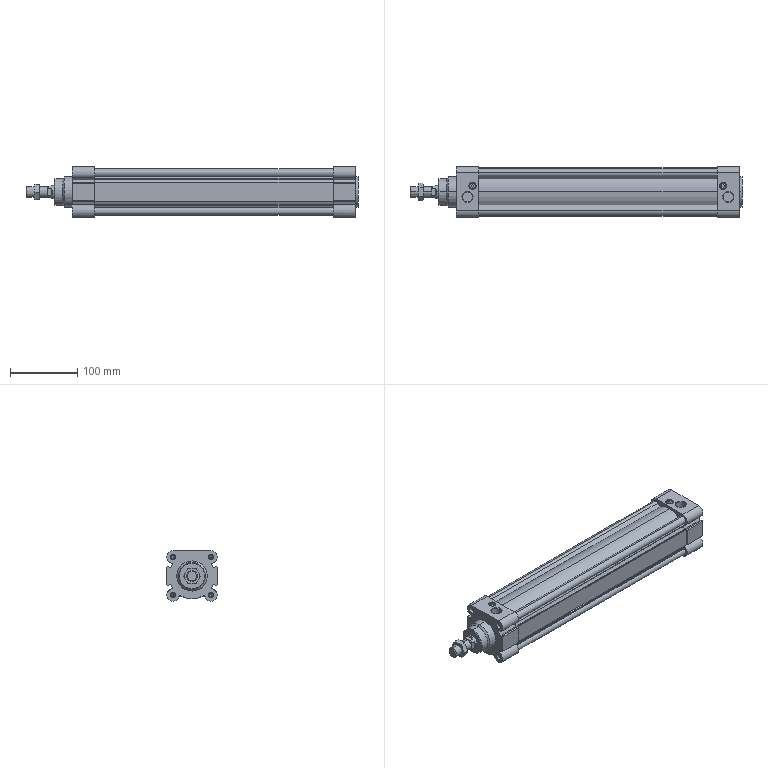Part | STEP file | 3 solids | 313 faces | box 494 x 75 x 75 mm | volume 957901 mm3 | plane 154 | cylinder 89 | cone 70 | commonest cylinder face diameters 4.917 x16 8.5 x16 4 x8 18.5 x8 12 x6 9.5 x4